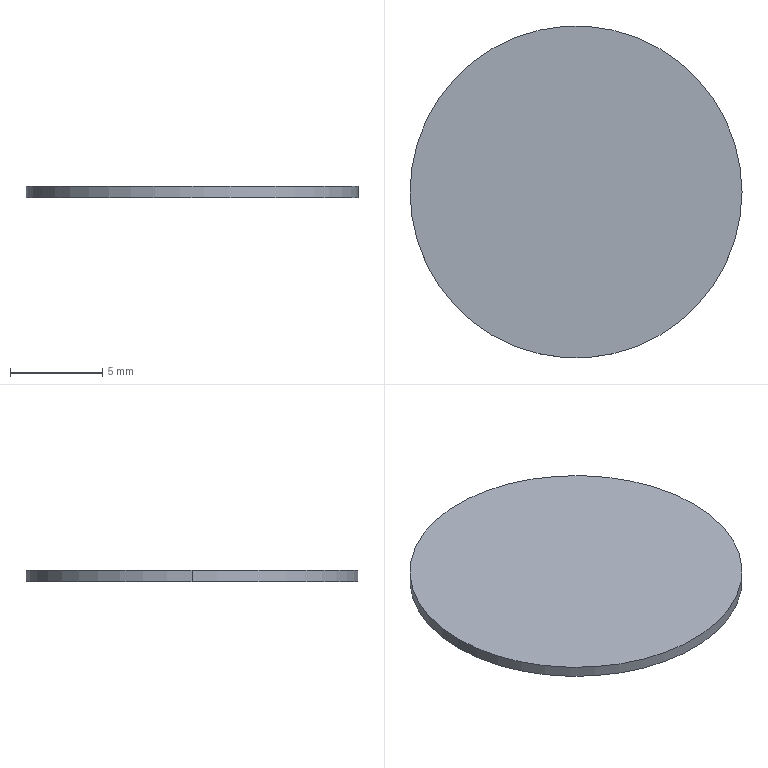Part | STEP file | 2023_07_21_12_39_19_0126 | 1 solid | 4 faces | box 18 x 18 x 0.6 mm | volume 152.681 mm3 | cylinder 2 | plane 2 | commonest cylinder face diameters 18 x2
STEP:
#1=CARTESIAN_POINT('',(6.5,81.,36.1));
#2=VERTEX_POINT('',#1);
#3=CARTESIAN_POINT('',(24.5,81.,36.1));
#4=VERTEX_POINT('',#3);
#5=CARTESIAN_POINT('',(15.5,81.,36.1));
#6=DIRECTION('',(0.,0.,1.));
#7=DIRECTION('',(1.,0.,0.));
#8=AXIS2_PLACEMENT_3D('',#5,#6,#7);
#9=CIRCLE('',#8,9.);
#10=EDGE_CURVE('',#2,#4,#9,.T.);
#11=ORIENTED_EDGE('',*,*,#10,.F.);
#12=CARTESIAN_POINT('',(6.5,81.,35.5));
#13=VERTEX_POINT('',#12);
#14=CARTESIAN_POINT('',(6.5,81.,35.8));
#15=DIRECTION('',(0.,0.,-1.));
#16=VECTOR('',#15,1000.);
#17=LINE('',#14,#16);
#18=EDGE_CURVE('',#2,#13,#17,.T.);
#19=ORIENTED_EDGE('',*,*,#18,.T.);
#20=CARTESIAN_POINT('',(24.5,81.,35.5));
#21=VERTEX_POINT('',#20);
#22=CARTESIAN_POINT('',(15.5,81.,35.5));
#23=DIRECTION('',(0.,0.,-1.));
#24=DIRECTION('',(1.,0.,0.));
#25=AXIS2_PLACEMENT_3D('',#22,#23,#24);
#26=CIRCLE('',#25,9.);
#27=EDGE_CURVE('',#21,#13,#26,.T.);
#28=ORIENTED_EDGE('',*,*,#27,.F.);
#29=CARTESIAN_POINT('',(24.5,81.,35.8));
#30=DIRECTION('',(0.,0.,-1.));
#31=VECTOR('',#30,1000.);
#32=LINE('',#29,#31);
#33=EDGE_CURVE('',#4,#21,#32,.T.);
#34=ORIENTED_EDGE('',*,*,#33,.F.);
#35=EDGE_LOOP('',(#11,#19,#28,#34));
#36=FACE_OUTER_BOUND('',#35,.T.);
#37=CARTESIAN_POINT('',(15.5,81.,35.8));
#38=DIRECTION('',(0.,0.,-1.));
#39=DIRECTION('',(1.,0.,0.));
#40=AXIS2_PLACEMENT_3D('',#37,#38,#39);
#41=CYLINDRICAL_SURFACE('',#40,9.);
#42=ADVANCED_FACE('',(#36),#41,.T.);
#43=CARTESIAN_POINT('',(15.5,81.,36.1));
#44=DIRECTION('',(0.,0.,1.));
#45=DIRECTION('',(1.,0.,0.));
#46=AXIS2_PLACEMENT_3D('',#43,#44,#45);
#47=CIRCLE('',#46,9.);
#48=EDGE_CURVE('',#4,#2,#47,.T.);
#49=ORIENTED_EDGE('',*,*,#48,.T.);
#50=ORIENTED_EDGE('',*,*,#10,.T.);
#51=EDGE_LOOP('',(#49,#50));
#52=FACE_OUTER_BOUND('',#51,.T.);
#53=CARTESIAN_POINT('',(15.5,81.,36.1));
#54=DIRECTION('',(0.,0.,1.));
#55=DIRECTION('',(1.,0.,0.));
#56=AXIS2_PLACEMENT_3D('',#53,#54,#55);
#57=PLANE('',#56);
#58=ADVANCED_FACE('',(#52),#57,.T.);
#59=ORIENTED_EDGE('',*,*,#27,.T.);
#60=CARTESIAN_POINT('',(15.5,81.,35.5));
#61=DIRECTION('',(0.,0.,-1.));
#62=DIRECTION('',(1.,0.,0.));
#63=AXIS2_PLACEMENT_3D('',#60,#61,#62);
#64=CIRCLE('',#63,9.);
#65=EDGE_CURVE('',#13,#21,#64,.T.);
#66=ORIENTED_EDGE('',*,*,#65,.T.);
#67=EDGE_LOOP('',(#59,#66));
#68=FACE_OUTER_BOUND('',#67,.T.);
#69=CARTESIAN_POINT('',(15.5,81.,35.5));
#70=DIRECTION('',(0.,0.,-1.));
#71=DIRECTION('',(0.,-1.,0.));
#72=AXIS2_PLACEMENT_3D('',#69,#70,#71);
#73=PLANE('',#72);
#74=ADVANCED_FACE('',(#68),#73,.T.);
#75=ORIENTED_EDGE('',*,*,#18,.F.);
#76=ORIENTED_EDGE('',*,*,#48,.F.);
#77=ORIENTED_EDGE('',*,*,#33,.T.);
#78=ORIENTED_EDGE('',*,*,#65,.F.);
#79=EDGE_LOOP('',(#75,#76,#77,#78));
#80=FACE_OUTER_BOUND('',#79,.T.);
#81=CARTESIAN_POINT('',(15.5,81.,35.8));
#82=DIRECTION('',(0.,0.,-1.));
#83=DIRECTION('',(1.,0.,0.));
#84=AXIS2_PLACEMENT_3D('',#81,#82,#83);
#85=CYLINDRICAL_SURFACE('',#84,9.);
#86=ADVANCED_FACE('',(#80),#85,.T.);
#87=CLOSED_SHELL('',(#42,#58,#74,#86));
#88=MANIFOLD_SOLID_BREP('',#87);
#89=CARTESIAN_POINT('',(0.,0.,0.));
#90=DIRECTION('',(0.,0.,1.));
#91=DIRECTION('',(1.,0.,0.));
#92=AXIS2_PLACEMENT_3D('',#89,#90,#91);
#93=(LENGTH_UNIT()NAMED_UNIT(*)SI_UNIT(.MILLI.,.METRE.));
#94=UNCERTAINTY_MEASURE_WITH_UNIT(LENGTH_MEASURE(0.00001),#93,'','');
#95=(NAMED_UNIT(*)PLANE_ANGLE_UNIT()SI_UNIT($,.RADIAN.));
#96=(NAMED_UNIT(*)SI_UNIT($,.STERADIAN.)SOLID_ANGLE_UNIT());
#97=(GEOMETRIC_REPRESENTATION_CONTEXT(3)GLOBAL_UNCERTAINTY_ASSIGNED_CONTEXT((#94))GLOBAL_UNIT_ASSIGNED_CONTEXT((#93,#95,#96))REPRESENTATION_CONTEXT('',''));
#98=ADVANCED_BREP_SHAPE_REPRESENTATION('',(#88,#92),#97);